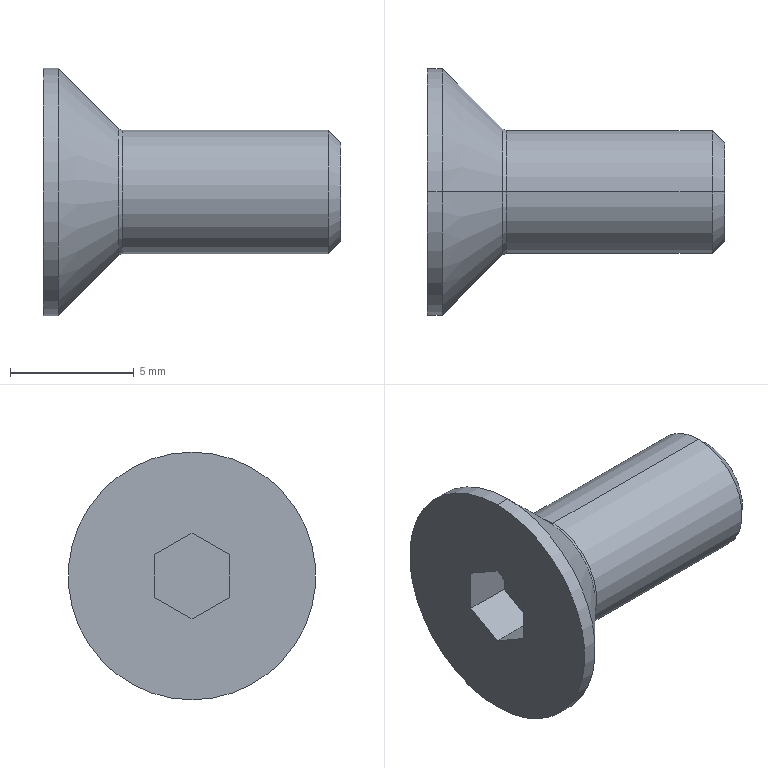Part | STEP file | 1 solid | 19 faces | box 12 x 10 x 10 mm | volume 319.784 mm3 | plane 9 | cone 4 | cylinder 4 | spline 2 | commonest cylinder face diameters 5 x2 10 x2
STEP:
#1=CARTESIAN_POINT('',(0.,0.,0.));
#2=DIRECTION('',(0.,0.,1.));
#3=DIRECTION('',(1.,0.,0.));
#4=AXIS2_PLACEMENT_3D('',#1,#2,#3);
#5=CARTESIAN_POINT('',(8.9,0.,2.));
#6=VERTEX_POINT('',#5);
#7=CARTESIAN_POINT('',(8.9,0.,-2.));
#8=VERTEX_POINT('',#7);
#9=CARTESIAN_POINT('',(8.9,0.,0.));
#10=DIRECTION('',(-1.,0.,0.));
#11=DIRECTION('',(0.,0.,1.));
#12=AXIS2_PLACEMENT_3D('',#9,#10,#11);
#13=CIRCLE('',#12,2.);
#14=CARTESIAN_POINT('',(8.9,2.5,0.));
#15=DIRECTION('',(-1.,0.,0.));
#16=DIRECTION('',(0.,0.,1.));
#17=AXIS2_PLACEMENT_3D('',#14,#15,#16);
#18=PLANE('',#17);
#19=CARTESIAN_POINT('',(0.,-2.5));
#20=DIRECTION('',(1.,0.));
#21=AXIS2_PLACEMENT_2D('',#19,#20);
#22=CIRCLE('',#21,2.);
#23=(GEOMETRIC_REPRESENTATION_CONTEXT(2)PARAMETRIC_REPRESENTATION_CONTEXT()REPRESENTATION_CONTEXT('',''));
#24=DEFINITIONAL_REPRESENTATION('',(#22),#23);
#25=PCURVE('',#18,#24);
#26=CARTESIAN_POINT('',(8.4,0.,0.));
#27=DIRECTION('',(-1.,0.,0.));
#28=DIRECTION('',(0.,0.,1.));
#29=AXIS2_PLACEMENT_3D('',#26,#27,#28);
#30=CONICAL_SURFACE('',#29,2.5,0.7854);
#31=CARTESIAN_POINT('',(0.,-0.5));
#32=DIRECTION('',(1.,0.));
#33=VECTOR('',#32,1.);
#34=LINE('',#31,#33);
#35=(GEOMETRIC_REPRESENTATION_CONTEXT(2)PARAMETRIC_REPRESENTATION_CONTEXT()REPRESENTATION_CONTEXT('',''));
#36=DEFINITIONAL_REPRESENTATION('',(#34),#35);
#37=PCURVE('',#30,#36);
#38=SURFACE_CURVE('',#13,(#25,#37),.PCURVE_S1.);
#39=EDGE_CURVE('',#6,#8,#38,.T.);
#40=ORIENTED_EDGE('',*,*,#39,.F.);
#41=CARTESIAN_POINT('',(8.9,0.,0.));
#42=DIRECTION('',(-1.,0.,0.));
#43=DIRECTION('',(0.,0.,1.));
#44=AXIS2_PLACEMENT_3D('',#41,#42,#43);
#45=CIRCLE('',#44,2.);
#46=CARTESIAN_POINT('',(0.,-2.5));
#47=DIRECTION('',(1.,0.));
#48=AXIS2_PLACEMENT_2D('',#46,#47);
#49=CIRCLE('',#48,2.);
#50=(GEOMETRIC_REPRESENTATION_CONTEXT(2)PARAMETRIC_REPRESENTATION_CONTEXT()REPRESENTATION_CONTEXT('',''));
#51=DEFINITIONAL_REPRESENTATION('',(#49),#50);
#52=PCURVE('',#18,#51);
#53=CARTESIAN_POINT('',(8.4,0.,0.));
#54=DIRECTION('',(-1.,0.,0.));
#55=DIRECTION('',(0.,0.,1.));
#56=AXIS2_PLACEMENT_3D('',#53,#54,#55);
#57=CONICAL_SURFACE('',#56,2.5,0.7854);
#58=CARTESIAN_POINT('',(0.,-0.5));
#59=DIRECTION('',(1.,0.));
#60=VECTOR('',#59,1.);
#61=LINE('',#58,#60);
#62=(GEOMETRIC_REPRESENTATION_CONTEXT(2)PARAMETRIC_REPRESENTATION_CONTEXT()REPRESENTATION_CONTEXT('',''));
#63=DEFINITIONAL_REPRESENTATION('',(#61),#62);
#64=PCURVE('',#57,#63);
#65=SURFACE_CURVE('',#45,(#52,#64),.PCURVE_S1.);
#66=EDGE_CURVE('',#8,#6,#65,.T.);
#67=ORIENTED_EDGE('',*,*,#66,.F.);
#68=EDGE_LOOP('',(#40,#67));
#69=FACE_BOUND('',#68,.T.);
#70=ADVANCED_FACE('',(#69),#18,.F.);
#71=CARTESIAN_POINT('',(8.4,0.,-2.5));
#72=VERTEX_POINT('',#71);
#73=CARTESIAN_POINT('',(8.4,0.,-2.5));
#74=DIRECTION('',(-0.7071,0.,-0.7071));
#75=VECTOR('',#74,1.);
#76=LINE('',#73,#75);
#77=CARTESIAN_POINT('',(3.142,0.));
#78=DIRECTION('',(0.,1.));
#79=VECTOR('',#78,1.);
#80=LINE('',#77,#79);
#81=(GEOMETRIC_REPRESENTATION_CONTEXT(2)PARAMETRIC_REPRESENTATION_CONTEXT()REPRESENTATION_CONTEXT('',''));
#82=DEFINITIONAL_REPRESENTATION('',(#80),#81);
#83=PCURVE('',#57,#82);
#84=CARTESIAN_POINT('',(3.142,0.));
#85=DIRECTION('',(0.,1.));
#86=VECTOR('',#85,1.);
#87=LINE('',#84,#86);
#88=(GEOMETRIC_REPRESENTATION_CONTEXT(2)PARAMETRIC_REPRESENTATION_CONTEXT()REPRESENTATION_CONTEXT('',''));
#89=DEFINITIONAL_REPRESENTATION('',(#87),#88);
#90=PCURVE('',#30,#89);
#91=SURFACE_CURVE('',#76,(#83,#90),.PCURVE_S1.);
#92=EDGE_CURVE('',#8,#72,#91,.T.);
#93=ORIENTED_EDGE('',*,*,#92,.F.);
#94=ORIENTED_EDGE('',*,*,#66,.T.);
#95=CARTESIAN_POINT('',(8.4,0.,2.5));
#96=VERTEX_POINT('',#95);
#97=CARTESIAN_POINT('',(8.4,0.,2.5));
#98=DIRECTION('',(-0.7071,0.,0.7071));
#99=VECTOR('',#98,1.);
#100=LINE('',#97,#99);
#101=CARTESIAN_POINT('',(6.283,0.));
#102=DIRECTION('',(0.,1.));
#103=VECTOR('',#102,1.);
#104=LINE('',#101,#103);
#105=(GEOMETRIC_REPRESENTATION_CONTEXT(2)PARAMETRIC_REPRESENTATION_CONTEXT()REPRESENTATION_CONTEXT('',''));
#106=DEFINITIONAL_REPRESENTATION('',(#104),#105);
#107=PCURVE('',#57,#106);
#108=CARTESIAN_POINT('',(0.,0.));
#109=DIRECTION('',(0.,1.));
#110=VECTOR('',#109,1.);
#111=LINE('',#108,#110);
#112=(GEOMETRIC_REPRESENTATION_CONTEXT(2)PARAMETRIC_REPRESENTATION_CONTEXT()REPRESENTATION_CONTEXT('',''));
#113=DEFINITIONAL_REPRESENTATION('',(#111),#112);
#114=PCURVE('',#30,#113);
#115=SURFACE_CURVE('',#100,(#107,#114),.PCURVE_S1.);
#116=EDGE_CURVE('',#6,#96,#115,.T.);
#117=ORIENTED_EDGE('',*,*,#116,.T.);
#118=CARTESIAN_POINT('',(8.4,0.,0.));
#119=DIRECTION('',(-1.,0.,0.));
#120=DIRECTION('',(0.,0.,1.));
#121=AXIS2_PLACEMENT_3D('',#118,#119,#120);
#122=CIRCLE('',#121,2.5);
#123=CARTESIAN_POINT('',(0.,0.));
#124=DIRECTION('',(1.,0.));
#125=VECTOR('',#124,1.);
#126=LINE('',#123,#125);
#127=(GEOMETRIC_REPRESENTATION_CONTEXT(2)PARAMETRIC_REPRESENTATION_CONTEXT()REPRESENTATION_CONTEXT('',''));
#128=DEFINITIONAL_REPRESENTATION('',(#126),#127);
#129=PCURVE('',#57,#128);
#130=CARTESIAN_POINT('',(-20.912,0.,0.));
#131=DIRECTION('',(-1.,0.,0.));
#132=DIRECTION('',(0.,0.,1.));
#133=AXIS2_PLACEMENT_3D('',#130,#131,#132);
#134=CYLINDRICAL_SURFACE('',#133,2.5);
#135=CARTESIAN_POINT('',(0.,-29.312));
#136=DIRECTION('',(1.,0.));
#137=VECTOR('',#136,1.);
#138=LINE('',#135,#137);
#139=(GEOMETRIC_REPRESENTATION_CONTEXT(2)PARAMETRIC_REPRESENTATION_CONTEXT()REPRESENTATION_CONTEXT('',''));
#140=DEFINITIONAL_REPRESENTATION('',(#138),#139);
#141=PCURVE('',#134,#140);
#142=SURFACE_CURVE('',#122,(#129,#141),.PCURVE_S1.);
#143=EDGE_CURVE('',#72,#96,#142,.T.);
#144=ORIENTED_EDGE('',*,*,#143,.F.);
#145=EDGE_LOOP('',(#93,#94,#117,#144));
#146=FACE_BOUND('',#145,.T.);
#147=ADVANCED_FACE('',(#146),#57,.T.);
#148=CARTESIAN_POINT('',(-3.1,-1.5,0.866));
#149=VERTEX_POINT('',#148);
#150=CARTESIAN_POINT('',(-1.2,-1.5,0.866));
#151=VERTEX_POINT('',#150);
#152=CARTESIAN_POINT('',(-1.2,-1.5,0.866));
#153=DIRECTION('',(1.,0.,0.));
#154=VECTOR('',#153,1.);
#155=LINE('',#152,#154);
#156=CARTESIAN_POINT('',(-1.2,-1.5,-0.866));
#157=DIRECTION('',(0.,-1.,0.));
#158=DIRECTION('',(-1.,0.,0.));
#159=AXIS2_PLACEMENT_3D('',#156,#157,#158);
#160=PLANE('',#159);
#161=CARTESIAN_POINT('',(0.,-1.732));
#162=DIRECTION('',(-1.,0.));
#163=VECTOR('',#162,1.);
#164=LINE('',#161,#163);
#165=(GEOMETRIC_REPRESENTATION_CONTEXT(2)PARAMETRIC_REPRESENTATION_CONTEXT()REPRESENTATION_CONTEXT('',''));
#166=DEFINITIONAL_REPRESENTATION('',(#164),#165);
#167=PCURVE('',#160,#166);
#168=CARTESIAN_POINT('',(-1.2,-1.5,0.866));
#169=DIRECTION('',(0.,-0.5,0.866));
#170=DIRECTION('',(-1.,0.,0.));
#171=AXIS2_PLACEMENT_3D('',#168,#169,#170);
#172=PLANE('',#171);
#173=CARTESIAN_POINT('',(0.,0.));
#174=DIRECTION('',(-1.,0.));
#175=VECTOR('',#174,1.);
#176=LINE('',#173,#175);
#177=(GEOMETRIC_REPRESENTATION_CONTEXT(2)PARAMETRIC_REPRESENTATION_CONTEXT()REPRESENTATION_CONTEXT('',''));
#178=DEFINITIONAL_REPRESENTATION('',(#176),#177);
#179=PCURVE('',#172,#178);
#180=SURFACE_CURVE('',#155,(#167,#179),.PCURVE_S1.);
#181=EDGE_CURVE('',#149,#151,#180,.T.);
#182=ORIENTED_EDGE('',*,*,#181,.T.);
#183=CARTESIAN_POINT('',(-1.2,-1.5,-0.866));
#184=VERTEX_POINT('',#183);
#185=CARTESIAN_POINT('',(-1.2,-1.5,-0.866));
#186=DIRECTION('',(0.,0.,1.));
#187=VECTOR('',#186,1.);
#188=LINE('',#185,#187);
#189=CARTESIAN_POINT('',(0.,0.));
#190=DIRECTION('',(0.,-1.));
#191=VECTOR('',#190,1.);
#192=LINE('',#189,#191);
#193=(GEOMETRIC_REPRESENTATION_CONTEXT(2)PARAMETRIC_REPRESENTATION_CONTEXT()REPRESENTATION_CONTEXT('',''));
#194=DEFINITIONAL_REPRESENTATION('',(#192),#193);
#195=PCURVE('',#160,#194);
#196=CARTESIAN_POINT('',(-1.2,0.,0.));
#197=DIRECTION('',(-1.,0.,0.));
#198=DIRECTION('',(0.,0.,1.));
#199=AXIS2_PLACEMENT_3D('',#196,#197,#198);
#200=PLANE('',#199);
#201=CARTESIAN_POINT('',(-0.866,-1.5));
#202=DIRECTION('',(1.,0.));
#203=VECTOR('',#202,1.);
#204=LINE('',#201,#203);
#205=(GEOMETRIC_REPRESENTATION_CONTEXT(2)PARAMETRIC_REPRESENTATION_CONTEXT()REPRESENTATION_CONTEXT('',''));
#206=DEFINITIONAL_REPRESENTATION('',(#204),#205);
#207=PCURVE('',#200,#206);
#208=SURFACE_CURVE('',#188,(#195,#207),.PCURVE_S1.);
#209=EDGE_CURVE('',#184,#151,#208,.T.);
#210=ORIENTED_EDGE('',*,*,#209,.F.);
#211=CARTESIAN_POINT('',(-3.1,-1.5,-0.866));
#212=VERTEX_POINT('',#211);
#213=CARTESIAN_POINT('',(-1.2,-1.5,-0.866));
#214=DIRECTION('',(-1.,0.,0.));
#215=VECTOR('',#214,1.);
#216=LINE('',#213,#215);
#217=CARTESIAN_POINT('',(0.,0.));
#218=DIRECTION('',(1.,0.));
#219=VECTOR('',#218,1.);
#220=LINE('',#217,#219);
#221=(GEOMETRIC_REPRESENTATION_CONTEXT(2)PARAMETRIC_REPRESENTATION_CONTEXT()REPRESENTATION_CONTEXT('',''));
#222=DEFINITIONAL_REPRESENTATION('',(#220),#221);
#223=PCURVE('',#160,#222);
#224=CARTESIAN_POINT('',(-1.2,0.,-1.732));
#225=DIRECTION('',(0.,-0.5,-0.866));
#226=DIRECTION('',(0.,-0.866,0.5));
#227=AXIS2_PLACEMENT_3D('',#224,#225,#226);
#228=PLANE('',#227);
#229=CARTESIAN_POINT('',(1.732,0.));
#230=DIRECTION('',(0.,1.));
#231=VECTOR('',#230,1.);
#232=LINE('',#229,#231);
#233=(GEOMETRIC_REPRESENTATION_CONTEXT(2)PARAMETRIC_REPRESENTATION_CONTEXT()REPRESENTATION_CONTEXT('',''));
#234=DEFINITIONAL_REPRESENTATION('',(#232),#233);
#235=PCURVE('',#228,#234);
#236=SURFACE_CURVE('',#216,(#223,#235),.PCURVE_S1.);
#237=EDGE_CURVE('',#184,#212,#236,.T.);
#238=ORIENTED_EDGE('',*,*,#237,.T.);
#239=CARTESIAN_POINT('',(-3.1,-1.5,-0.866));
#240=DIRECTION('',(0.,0.,-1.));
#241=VECTOR('',#240,1.);
#242=LINE('',#239,#241);
#243=CARTESIAN_POINT('',(1.9,0.));
#244=DIRECTION('',(0.,1.));
#245=VECTOR('',#244,1.);
#246=LINE('',#243,#245);
#247=(GEOMETRIC_REPRESENTATION_CONTEXT(2)PARAMETRIC_REPRESENTATION_CONTEXT()REPRESENTATION_CONTEXT('',''));
#248=DEFINITIONAL_REPRESENTATION('',(#246),#247);
#249=PCURVE('',#160,#248);
#250=CARTESIAN_POINT('',(-3.1,5.,0.));
#251=DIRECTION('',(1.,0.,0.));
#252=DIRECTION('',(0.,1.,0.));
#253=AXIS2_PLACEMENT_3D('',#250,#251,#252);
#254=PLANE('',#253);
#255=CARTESIAN_POINT('',(-6.5,-0.866));
#256=DIRECTION('',(0.,-1.));
#257=VECTOR('',#256,1.);
#258=LINE('',#255,#257);
#259=(GEOMETRIC_REPRESENTATION_CONTEXT(2)PARAMETRIC_REPRESENTATION_CONTEXT()REPRESENTATION_CONTEXT('',''));
#260=DEFINITIONAL_REPRESENTATION('',(#258),#259);
#261=PCURVE('',#254,#260);
#262=SURFACE_CURVE('',#242,(#249,#261),.PCURVE_S1.);
#263=EDGE_CURVE('',#149,#212,#262,.T.);
#264=ORIENTED_EDGE('',*,*,#263,.F.);
#265=EDGE_LOOP('',(#182,#210,#238,#264));
#266=FACE_BOUND('',#265,.T.);
#267=ADVANCED_FACE('',(#266),#160,.F.);
#268=CARTESIAN_POINT('',(0.08284,0.,-2.5));
#269=VERTEX_POINT('',#268);
#270=CARTESIAN_POINT('',(-20.912,0.,-2.5));
#271=DIRECTION('',(-1.,0.,0.));
#272=VECTOR('',#271,1.);
#273=LINE('',#270,#272);
#274=CARTESIAN_POINT('',(3.142,0.));
#275=DIRECTION('',(0.,1.));
#276=VECTOR('',#275,1.);
#277=LINE('',#274,#276);
#278=(GEOMETRIC_REPRESENTATION_CONTEXT(2)PARAMETRIC_REPRESENTATION_CONTEXT()REPRESENTATION_CONTEXT('',''));
#279=DEFINITIONAL_REPRESENTATION('',(#277),#278);
#280=PCURVE('',#134,#279);
#281=CARTESIAN_POINT('',(-20.912,0.,0.));
#282=DIRECTION('',(-1.,0.,0.));
#283=DIRECTION('',(0.,0.,1.));
#284=AXIS2_PLACEMENT_3D('',#281,#282,#283);
#285=CYLINDRICAL_SURFACE('',#284,2.5);
#286=CARTESIAN_POINT('',(3.142,0.));
#287=DIRECTION('',(0.,1.));
#288=VECTOR('',#287,1.);
#289=LINE('',#286,#288);
#290=(GEOMETRIC_REPRESENTATION_CONTEXT(2)PARAMETRIC_REPRESENTATION_CONTEXT()REPRESENTATION_CONTEXT('',''));
#291=DEFINITIONAL_REPRESENTATION('',(#289),#290);
#292=PCURVE('',#285,#291);
#293=SURFACE_CURVE('',#273,(#280,#292),.PCURVE_S1.);
#294=EDGE_CURVE('',#72,#269,#293,.T.);
#295=ORIENTED_EDGE('',*,*,#294,.F.);
#296=ORIENTED_EDGE('',*,*,#143,.T.);
#297=CARTESIAN_POINT('',(0.08284,0.,2.5));
#298=VERTEX_POINT('',#297);
#299=CARTESIAN_POINT('',(-20.912,0.,2.5));
#300=DIRECTION('',(-1.,0.,0.));
#301=VECTOR('',#300,1.);
#302=LINE('',#299,#301);
#303=CARTESIAN_POINT('',(6.283,0.));
#304=DIRECTION('',(0.,1.));
#305=VECTOR('',#304,1.);
#306=LINE('',#303,#305);
#307=(GEOMETRIC_REPRESENTATION_CONTEXT(2)PARAMETRIC_REPRESENTATION_CONTEXT()REPRESENTATION_CONTEXT('',''));
#308=DEFINITIONAL_REPRESENTATION('',(#306),#307);
#309=PCURVE('',#134,#308);
#310=CARTESIAN_POINT('',(0.,0.));
#311=DIRECTION('',(0.,1.));
#312=VECTOR('',#311,1.);
#313=LINE('',#310,#312);
#314=(GEOMETRIC_REPRESENTATION_CONTEXT(2)PARAMETRIC_REPRESENTATION_CONTEXT()REPRESENTATION_CONTEXT('',''));
#315=DEFINITIONAL_REPRESENTATION('',(#313),#314);
#316=PCURVE('',#285,#315);
#317=SURFACE_CURVE('',#302,(#309,#316),.PCURVE_S1.);
#318=EDGE_CURVE('',#96,#298,#317,.T.);
#319=ORIENTED_EDGE('',*,*,#318,.T.);
#320=CARTESIAN_POINT('',(0.08284,0.,0.));
#321=DIRECTION('',(1.,0.,0.));
#322=DIRECTION('',(0.,0.,1.));
#323=AXIS2_PLACEMENT_3D('',#320,#321,#322);
#324=CIRCLE('',#323,2.5);
#325=CARTESIAN_POINT('',(6.283,-20.995));
#326=DIRECTION('',(-1.,0.));
#327=VECTOR('',#326,1.);
#328=LINE('',#325,#327);
#329=(GEOMETRIC_REPRESENTATION_CONTEXT(2)PARAMETRIC_REPRESENTATION_CONTEXT()REPRESENTATION_CONTEXT('',''));
#330=DEFINITIONAL_REPRESENTATION('',(#328),#329);
#331=PCURVE('',#134,#330);
#332=CARTESIAN_POINT('',(0.08284,0.,-2.5));
#333=CARTESIAN_POINT('',(0.08284,-5.,-2.5));
#334=CARTESIAN_POINT('',(0.08284,-5.,2.5));
#335=CARTESIAN_POINT('',(0.08284,0.,2.5));
#336=CARTESIAN_POINT('',(0.02909,0.,-2.5));
#337=CARTESIAN_POINT('',(0.02909,-5.,-2.5));
#338=CARTESIAN_POINT('',(0.02909,-5.,2.5));
#339=CARTESIAN_POINT('',(0.02909,0.,2.5));
#340=CARTESIAN_POINT('',(-0.02057,0.,-2.521));
#341=CARTESIAN_POINT('',(-0.02057,-5.041,-2.521));
#342=CARTESIAN_POINT('',(-0.02057,-5.041,2.521));
#343=CARTESIAN_POINT('',(-0.02057,0.,2.521));
#344=CARTESIAN_POINT('',(-0.05858,0.,-2.559));
#345=CARTESIAN_POINT('',(-0.05858,-5.117,-2.559));
#346=CARTESIAN_POINT('',(-0.05858,-5.117,2.559));
#347=CARTESIAN_POINT('',(-0.05858,0.,2.559));
#348=(BOUNDED_SURFACE()B_SPLINE_SURFACE(3,3,((#332,#333,#334,#335),(#336,#337,#338,#339),(#340,#341,#342,#343),(#344,#345,#346,#347)),.UNSPECIFIED.,.F.,.F.,.F.)B_SPLINE_SURFACE_WITH_KNOTS((4,4),(4,4),(0.,1.),(0.,1.),.PIECEWISE_BEZIER_KNOTS.)GEOMETRIC_REPRESENTATION_ITEM()RATIONAL_B_SPLINE_SURFACE(((1.,0.3333,0.3333,1.),(0.9493,0.3164,0.3164,0.9493),(0.9493,0.3164,0.3164,0.9493),(1.,0.3333,0.3333,1.)))REPRESENTATION_ITEM('')SURFACE());
#349=CARTESIAN_POINT('',(0.,1.));
#350=CARTESIAN_POINT('',(0.,0.9763));
#351=CARTESIAN_POINT('',(0.,0.9319));
#352=CARTESIAN_POINT('',(0.,0.8733));
#353=CARTESIAN_POINT('',(0.,0.8206));
#354=CARTESIAN_POINT('',(0.,0.7724));
#355=CARTESIAN_POINT('',(0.,0.7279));
#356=CARTESIAN_POINT('',(0.,0.6861));
#357=CARTESIAN_POINT('',(0.,0.6465));
#358=CARTESIAN_POINT('',(0.,0.6086));
#359=CARTESIAN_POINT('',(0.,0.5718));
#360=CARTESIAN_POINT('',(0.,0.5357));
#361=CARTESIAN_POINT('',(0.,0.5));
#362=CARTESIAN_POINT('',(0.,0.4643));
#363=CARTESIAN_POINT('',(0.,0.4282));
#364=CARTESIAN_POINT('',(0.,0.3914));
#365=CARTESIAN_POINT('',(0.,0.3535));
#366=CARTESIAN_POINT('',(0.,0.3139));
#367=CARTESIAN_POINT('',(0.,0.2721));
#368=CARTESIAN_POINT('',(0.,0.2276));
#369=CARTESIAN_POINT('',(0.,0.1794));
#370=CARTESIAN_POINT('',(0.,0.1267));
#371=CARTESIAN_POINT('',(0.,0.06805));
#372=CARTESIAN_POINT('',(0.,0.02375));
#373=CARTESIAN_POINT('',(0.,0.));
#374=B_SPLINE_CURVE_WITH_KNOTS('',3,(#349,#350,#351,#352,#353,#354,#355,#356,#357,#358,#359,#360,#361,#362,#363,#364,#365,#366,#367,#368,#369,#370,#371,#372,#373),.UNSPECIFIED.,.F.,.F.,(4,1,1,1,1,1,1,1,1,1,1,1,1,1,1,1,1,1,1,1,1,1,4),(0.,0.1428,0.2856,0.4284,0.5712,0.714,0.8568,0.9996,1.142,1.285,1.428,1.571,1.714,1.856,1.999,2.142,2.285,2.428,2.57,2.713,2.856,2.999,3.142),.QUASI_UNIFORM_KNOTS.);
#375=(GEOMETRIC_REPRESENTATION_CONTEXT(2)PARAMETRIC_REPRESENTATION_CONTEXT()REPRESENTATION_CONTEXT('',''));
#376=DEFINITIONAL_REPRESENTATION('',(#374),#375);
#377=PCURVE('',#348,#376);
#378=SURFACE_CURVE('',#324,(#331,#377),.PCURVE_S1.);
#379=EDGE_CURVE('',#298,#269,#378,.T.);
#380=ORIENTED_EDGE('',*,*,#379,.T.);
#381=EDGE_LOOP('',(#295,#296,#319,#380));
#382=FACE_BOUND('',#381,.T.);
#383=ADVANCED_FACE('',(#382),#134,.T.);
#384=CARTESIAN_POINT('',(-3.1,0.,1.732));
#385=VERTEX_POINT('',#384);
#386=CARTESIAN_POINT('',(-1.2,0.,1.732));
#387=VERTEX_POINT('',#386);
#388=CARTESIAN_POINT('',(-1.2,0.,1.732));
#389=DIRECTION('',(1.,0.,0.));
#390=VECTOR('',#389,1.);
#391=LINE('',#388,#390);
#392=CARTESIAN_POINT('',(0.,-1.732));
#393=DIRECTION('',(-1.,0.));
#394=VECTOR('',#393,1.);
#395=LINE('',#392,#394);
#396=(GEOMETRIC_REPRESENTATION_CONTEXT(2)PARAMETRIC_REPRESENTATION_CONTEXT()REPRESENTATION_CONTEXT('',''));
#397=DEFINITIONAL_REPRESENTATION('',(#395),#396);
#398=PCURVE('',#172,#397);
#399=CARTESIAN_POINT('',(-1.2,0.,1.732));
#400=DIRECTION('',(0.,0.5,0.866));
#401=DIRECTION('',(1.,0.,0.));
#402=AXIS2_PLACEMENT_3D('',#399,#400,#401);
#403=PLANE('',#402);
#404=CARTESIAN_POINT('',(0.,0.));
#405=DIRECTION('',(1.,0.));
#406=VECTOR('',#405,1.);
#407=LINE('',#404,#406);
#408=(GEOMETRIC_REPRESENTATION_CONTEXT(2)PARAMETRIC_REPRESENTATION_CONTEXT()REPRESENTATION_CONTEXT('',''));
#409=DEFINITIONAL_REPRESENTATION('',(#407),#408);
#410=PCURVE('',#403,#409);
#411=SURFACE_CURVE('',#391,(#398,#410),.PCURVE_S1.);
#412=EDGE_CURVE('',#385,#387,#411,.T.);
#413=ORIENTED_EDGE('',*,*,#412,.T.);
#414=CARTESIAN_POINT('',(-1.2,-1.5,0.866));
#415=DIRECTION('',(0.,0.866,0.5));
#416=VECTOR('',#415,1.);
#417=LINE('',#414,#416);
#418=CARTESIAN_POINT('',(0.,0.));
#419=DIRECTION('',(0.,-1.));
#420=VECTOR('',#419,1.);
#421=LINE('',#418,#420);
#422=(GEOMETRIC_REPRESENTATION_CONTEXT(2)PARAMETRIC_REPRESENTATION_CONTEXT()REPRESENTATION_CONTEXT('',''));
#423=DEFINITIONAL_REPRESENTATION('',(#421),#422);
#424=PCURVE('',#172,#423);
#425=CARTESIAN_POINT('',(0.866,-1.5));
#426=DIRECTION('',(0.5,0.866));
#427=VECTOR('',#426,1.);
#428=LINE('',#425,#427);
#429=(GEOMETRIC_REPRESENTATION_CONTEXT(2)PARAMETRIC_REPRESENTATION_CONTEXT()REPRESENTATION_CONTEXT('',''));
#430=DEFINITIONAL_REPRESENTATION('',(#428),#429);
#431=PCURVE('',#200,#430);
#432=SURFACE_CURVE('',#417,(#424,#431),.PCURVE_S1.);
#433=EDGE_CURVE('',#151,#387,#432,.T.);
#434=ORIENTED_EDGE('',*,*,#433,.F.);
#435=ORIENTED_EDGE('',*,*,#181,.F.);
#436=CARTESIAN_POINT('',(-3.1,-1.5,0.866));
#437=DIRECTION('',(0.,-0.866,-0.5));
#438=VECTOR('',#437,1.);
#439=LINE('',#436,#438);
#440=CARTESIAN_POINT('',(1.9,0.));
#441=DIRECTION('',(0.,1.));
#442=VECTOR('',#441,1.);
#443=LINE('',#440,#442);
#444=(GEOMETRIC_REPRESENTATION_CONTEXT(2)PARAMETRIC_REPRESENTATION_CONTEXT()REPRESENTATION_CONTEXT('',''));
#445=DEFINITIONAL_REPRESENTATION('',(#443),#444);
#446=PCURVE('',#172,#445);
#447=CARTESIAN_POINT('',(-6.5,0.866));
#448=DIRECTION('',(-0.866,-0.5));
#449=VECTOR('',#448,1.);
#450=LINE('',#447,#449);
#451=(GEOMETRIC_REPRESENTATION_CONTEXT(2)PARAMETRIC_REPRESENTATION_CONTEXT()REPRESENTATION_CONTEXT('',''));
#452=DEFINITIONAL_REPRESENTATION('',(#450),#451);
#453=PCURVE('',#254,#452);
#454=SURFACE_CURVE('',#439,(#446,#453),.PCURVE_S1.);
#455=EDGE_CURVE('',#385,#149,#454,.T.);
#456=ORIENTED_EDGE('',*,*,#455,.F.);
#457=EDGE_LOOP('',(#413,#434,#435,#456));
#458=FACE_BOUND('',#457,.T.);
#459=ADVANCED_FACE('',(#458),#172,.F.);
#460=ORIENTED_EDGE('',*,*,#237,.F.);
#461=CARTESIAN_POINT('',(-1.2,0.,-1.732));
#462=VERTEX_POINT('',#461);
#463=CARTESIAN_POINT('',(-1.2,0.,-1.732));
#464=DIRECTION('',(0.,-0.866,0.5));
#465=VECTOR('',#464,1.);
#466=LINE('',#463,#465);
#467=CARTESIAN_POINT('',(0.,0.));
#468=DIRECTION('',(1.,0.));
#469=VECTOR('',#468,1.);
#470=LINE('',#467,#469);
#471=(GEOMETRIC_REPRESENTATION_CONTEXT(2)PARAMETRIC_REPRESENTATION_CONTEXT()REPRESENTATION_CONTEXT('',''));
#472=DEFINITIONAL_REPRESENTATION('',(#470),#471);
#473=PCURVE('',#228,#472);
#474=CARTESIAN_POINT('',(-1.732,0.));
#475=DIRECTION('',(0.5,-0.866));
#476=VECTOR('',#475,1.);
#477=LINE('',#474,#476);
#478=(GEOMETRIC_REPRESENTATION_CONTEXT(2)PARAMETRIC_REPRESENTATION_CONTEXT()REPRESENTATION_CONTEXT('',''));
#479=DEFINITIONAL_REPRESENTATION('',(#477),#478);
#480=PCURVE('',#200,#479);
#481=SURFACE_CURVE('',#466,(#473,#480),.PCURVE_S1.);
#482=EDGE_CURVE('',#462,#184,#481,.T.);
#483=ORIENTED_EDGE('',*,*,#482,.F.);
#484=CARTESIAN_POINT('',(-3.1,0.,-1.732));
#485=VERTEX_POINT('',#484);
#486=CARTESIAN_POINT('',(-1.2,0.,-1.732));
#487=DIRECTION('',(-1.,0.,0.));
#488=VECTOR('',#487,1.);
#489=LINE('',#486,#488);
#490=CARTESIAN_POINT('',(0.,0.));
#491=DIRECTION('',(0.,1.));
#492=VECTOR('',#491,1.);
#493=LINE('',#490,#492);
#494=(GEOMETRIC_REPRESENTATION_CONTEXT(2)PARAMETRIC_REPRESENTATION_CONTEXT()REPRESENTATION_CONTEXT('',''));
#495=DEFINITIONAL_REPRESENTATION('',(#493),#494);
#496=PCURVE('',#228,#495);
#497=CARTESIAN_POINT('',(-1.2,1.5,-0.866));
#498=DIRECTION('',(0.,0.5,-0.866));
#499=DIRECTION('',(-1.,0.,0.));
#500=AXIS2_PLACEMENT_3D('',#497,#498,#499);
#501=PLANE('',#500);
#502=CARTESIAN_POINT('',(0.,-1.732));
#503=DIRECTION('',(1.,0.));
#504=VECTOR('',#503,1.);
#505=LINE('',#502,#504);
#506=(GEOMETRIC_REPRESENTATION_CONTEXT(2)PARAMETRIC_REPRESENTATION_CONTEXT()REPRESENTATION_CONTEXT('',''));
#507=DEFINITIONAL_REPRESENTATION('',(#505),#506);
#508=PCURVE('',#501,#507);
#509=SURFACE_CURVE('',#489,(#496,#508),.PCURVE_S1.);
#510=EDGE_CURVE('',#462,#485,#509,.T.);
#511=ORIENTED_EDGE('',*,*,#510,.T.);
#512=CARTESIAN_POINT('',(-3.1,0.,-1.732));
#513=DIRECTION('',(0.,0.866,-0.5));
#514=VECTOR('',#513,1.);
#515=LINE('',#512,#514);
#516=CARTESIAN_POINT('',(0.,1.9));
#517=DIRECTION('',(-1.,0.));
#518=VECTOR('',#517,1.);
#519=LINE('',#516,#518);
#520=(GEOMETRIC_REPRESENTATION_CONTEXT(2)PARAMETRIC_REPRESENTATION_CONTEXT()REPRESENTATION_CONTEXT('',''));
#521=DEFINITIONAL_REPRESENTATION('',(#519),#520);
#522=PCURVE('',#228,#521);
#523=CARTESIAN_POINT('',(-5.,-1.732));
#524=DIRECTION('',(0.866,-0.5));
#525=VECTOR('',#524,1.);
#526=LINE('',#523,#525);
#527=(GEOMETRIC_REPRESENTATION_CONTEXT(2)PARAMETRIC_REPRESENTATION_CONTEXT()REPRESENTATION_CONTEXT('',''));
#528=DEFINITIONAL_REPRESENTATION('',(#526),#527);
#529=PCURVE('',#254,#528);
#530=SURFACE_CURVE('',#515,(#522,#529),.PCURVE_S1.);
#531=EDGE_CURVE('',#212,#485,#530,.T.);
#532=ORIENTED_EDGE('',*,*,#531,.F.);
#533=EDGE_LOOP('',(#460,#483,#511,#532));
#534=FACE_BOUND('',#533,.T.);
#535=ADVANCED_FACE('',(#534),#228,.F.);
#536=CARTESIAN_POINT('',(-0.05858,0.,-2.559));
#537=VERTEX_POINT('',#536);
#538=CARTESIAN_POINT('',(-0.05858,0.,2.559));
#539=VERTEX_POINT('',#538);
#540=CARTESIAN_POINT('',(-0.05858,0.,0.));
#541=DIRECTION('',(-1.,0.,0.));
#542=DIRECTION('',(0.,0.,1.));
#543=AXIS2_PLACEMENT_3D('',#540,#541,#542);
#544=CIRCLE('',#543,2.559);
#545=CARTESIAN_POINT('',(1.,0.));
#546=CARTESIAN_POINT('',(1.,0.02375));
#547=CARTESIAN_POINT('',(1.,0.06805));
#548=CARTESIAN_POINT('',(1.,0.1267));
#549=CARTESIAN_POINT('',(1.,0.1794));
#550=CARTESIAN_POINT('',(1.,0.2276));
#551=CARTESIAN_POINT('',(1.,0.2721));
#552=CARTESIAN_POINT('',(1.,0.3139));
#553=CARTESIAN_POINT('',(1.,0.3535));
#554=CARTESIAN_POINT('',(1.,0.3914));
#555=CARTESIAN_POINT('',(1.,0.4282));
#556=CARTESIAN_POINT('',(1.,0.4643));
#557=CARTESIAN_POINT('',(1.,0.5));
#558=CARTESIAN_POINT('',(1.,0.5357));
#559=CARTESIAN_POINT('',(1.,0.5718));
#560=CARTESIAN_POINT('',(1.,0.6086));
#561=CARTESIAN_POINT('',(1.,0.6465));
#562=CARTESIAN_POINT('',(1.,0.6861));
#563=CARTESIAN_POINT('',(1.,0.7279));
#564=CARTESIAN_POINT('',(1.,0.7724));
#565=CARTESIAN_POINT('',(1.,0.8206));
#566=CARTESIAN_POINT('',(1.,0.8733));
#567=CARTESIAN_POINT('',(1.,0.9319));
#568=CARTESIAN_POINT('',(1.,0.9763));
#569=CARTESIAN_POINT('',(1.,1.));
#570=B_SPLINE_CURVE_WITH_KNOTS('',3,(#545,#546,#547,#548,#549,#550,#551,#552,#553,#554,#555,#556,#557,#558,#559,#560,#561,#562,#563,#564,#565,#566,#567,#568,#569),.UNSPECIFIED.,.F.,.F.,(4,1,1,1,1,1,1,1,1,1,1,1,1,1,1,1,1,1,1,1,1,1,4),(3.142,3.284,3.427,3.57,3.713,3.856,3.998,4.141,4.284,4.427,4.57,4.712,4.855,4.998,5.141,5.284,5.426,5.569,5.712,5.855,5.998,6.14,6.283),.QUASI_UNIFORM_KNOTS.);
#571=(GEOMETRIC_REPRESENTATION_CONTEXT(2)PARAMETRIC_REPRESENTATION_CONTEXT()REPRESENTATION_CONTEXT('',''));
#572=DEFINITIONAL_REPRESENTATION('',(#570),#571);
#573=PCURVE('',#348,#572);
#574=CARTESIAN_POINT('',(-2.5,0.,0.));
#575=DIRECTION('',(-1.,0.,0.));
#576=DIRECTION('',(0.,0.,1.));
#577=AXIS2_PLACEMENT_3D('',#574,#575,#576);
#578=CONICAL_SURFACE('',#577,5.,0.7854);
#579=CARTESIAN_POINT('',(0.,-2.441));
#580=DIRECTION('',(1.,0.));
#581=VECTOR('',#580,1.);
#582=LINE('',#579,#581);
#583=(GEOMETRIC_REPRESENTATION_CONTEXT(2)PARAMETRIC_REPRESENTATION_CONTEXT()REPRESENTATION_CONTEXT('',''));
#584=DEFINITIONAL_REPRESENTATION('',(#582),#583);
#585=PCURVE('',#578,#584);
#586=SURFACE_CURVE('',#544,(#573,#585),.PCURVE_S1.);
#587=EDGE_CURVE('',#537,#539,#586,.T.);
#588=ORIENTED_EDGE('',*,*,#587,.T.);
#589=CARTESIAN_POINT('',(0.08284,0.,2.7));
#590=DIRECTION('',(0.,1.,0.));
#591=DIRECTION('',(0.,0.,1.));
#592=AXIS2_PLACEMENT_3D('',#589,#590,#591);
#593=CIRCLE('',#592,0.2);
#594=CARTESIAN_POINT('',(0.,1.));
#595=CARTESIAN_POINT('',(0.01555,1.));
#596=CARTESIAN_POINT('',(0.04653,1.));
#597=CARTESIAN_POINT('',(0.09271,1.));
#598=CARTESIAN_POINT('',(0.1386,1.));
#599=CARTESIAN_POINT('',(0.1843,1.));
#600=CARTESIAN_POINT('',(0.2298,1.));
#601=CARTESIAN_POINT('',(0.2751,1.));
#602=CARTESIAN_POINT('',(0.3202,1.));
#603=CARTESIAN_POINT('',(0.3653,1.));
#604=CARTESIAN_POINT('',(0.4102,1.));
#605=CARTESIAN_POINT('',(0.4551,1.));
#606=CARTESIAN_POINT('',(0.5,1.));
#607=CARTESIAN_POINT('',(0.5449,1.));
#608=CARTESIAN_POINT('',(0.5898,1.));
#609=CARTESIAN_POINT('',(0.6347,1.));
#610=CARTESIAN_POINT('',(0.6798,1.));
#611=CARTESIAN_POINT('',(0.7249,1.));
#612=CARTESIAN_POINT('',(0.7702,1.));
#613=CARTESIAN_POINT('',(0.8157,1.));
#614=CARTESIAN_POINT('',(0.8614,1.));
#615=CARTESIAN_POINT('',(0.9073,1.));
#616=CARTESIAN_POINT('',(0.9535,1.));
#617=CARTESIAN_POINT('',(0.9845,1.));
#618=CARTESIAN_POINT('',(1.,1.));
#619=B_SPLINE_CURVE_WITH_KNOTS('',3,(#594,#595,#596,#597,#598,#599,#600,#601,#602,#603,#604,#605,#606,#607,#608,#609,#610,#611,#612,#613,#614,#615,#616,#617,#618),.UNSPECIFIED.,.F.,.F.,(4,1,1,1,1,1,1,1,1,1,1,1,1,1,1,1,1,1,1,1,1,1,4),(3.142,3.177,3.213,3.249,3.284,3.32,3.356,3.391,3.427,3.463,3.499,3.534,3.57,3.606,3.641,3.677,3.713,3.748,3.784,3.82,3.856,3.891,3.927),.QUASI_UNIFORM_KNOTS.);
#620=(GEOMETRIC_REPRESENTATION_CONTEXT(2)PARAMETRIC_REPRESENTATION_CONTEXT()REPRESENTATION_CONTEXT('',''));
#621=DEFINITIONAL_REPRESENTATION('',(#619),#620);
#622=PCURVE('',#348,#621);
#623=CARTESIAN_POINT('',(0.08284,0.,2.5));
#624=CARTESIAN_POINT('',(0.08284,5.,2.5));
#625=CARTESIAN_POINT('',(0.08284,5.,-2.5));
#626=CARTESIAN_POINT('',(0.08284,0.,-2.5));
#627=CARTESIAN_POINT('',(0.02909,0.,2.5));
#628=CARTESIAN_POINT('',(0.02909,5.,2.5));
#629=CARTESIAN_POINT('',(0.02909,5.,-2.5));
#630=CARTESIAN_POINT('',(0.02909,0.,-2.5));
#631=CARTESIAN_POINT('',(-0.02057,0.,2.521));
#632=CARTESIAN_POINT('',(-0.02057,5.041,2.521));
#633=CARTESIAN_POINT('',(-0.02057,5.041,-2.521));
#634=CARTESIAN_POINT('',(-0.02057,0.,-2.521));
#635=CARTESIAN_POINT('',(-0.05858,0.,2.559));
#636=CARTESIAN_POINT('',(-0.05858,5.117,2.559));
#637=CARTESIAN_POINT('',(-0.05858,5.117,-2.559));
#638=CARTESIAN_POINT('',(-0.05858,0.,-2.559));
#639=(BOUNDED_SURFACE()B_SPLINE_SURFACE(3,3,((#623,#624,#625,#626),(#627,#628,#629,#630),(#631,#632,#633,#634),(#635,#636,#637,#638)),.UNSPECIFIED.,.F.,.F.,.F.)B_SPLINE_SURFACE_WITH_KNOTS((4,4),(4,4),(0.,1.),(0.,1.),.PIECEWISE_BEZIER_KNOTS.)GEOMETRIC_REPRESENTATION_ITEM()RATIONAL_B_SPLINE_SURFACE(((1.,0.3333,0.3333,1.),(0.9493,0.3164,0.3164,0.9493),(0.9493,0.3164,0.3164,0.9493),(1.,0.3333,0.3333,1.)))REPRESENTATION_ITEM('')SURFACE());
#640=CARTESIAN_POINT('',(0.,0.));
#641=CARTESIAN_POINT('',(0.01555,0.));
#642=CARTESIAN_POINT('',(0.04653,0.));
#643=CARTESIAN_POINT('',(0.09271,0.));
#644=CARTESIAN_POINT('',(0.1386,0.));
#645=CARTESIAN_POINT('',(0.1843,0.));
#646=CARTESIAN_POINT('',(0.2298,0.));
#647=CARTESIAN_POINT('',(0.2751,0.));
#648=CARTESIAN_POINT('',(0.3202,0.));
#649=CARTESIAN_POINT('',(0.3653,0.));
#650=CARTESIAN_POINT('',(0.4102,0.));
#651=CARTESIAN_POINT('',(0.4551,0.));
#652=CARTESIAN_POINT('',(0.5,0.));
#653=CARTESIAN_POINT('',(0.5449,0.));
#654=CARTESIAN_POINT('',(0.5898,0.));
#655=CARTESIAN_POINT('',(0.6347,0.));
#656=CARTESIAN_POINT('',(0.6798,0.));
#657=CARTESIAN_POINT('',(0.7249,0.));
#658=CARTESIAN_POINT('',(0.7702,0.));
#659=CARTESIAN_POINT('',(0.8157,0.));
#660=CARTESIAN_POINT('',(0.8614,0.));
#661=CARTESIAN_POINT('',(0.9073,0.));
#662=CARTESIAN_POINT('',(0.9535,0.));
#663=CARTESIAN_POINT('',(0.9845,0.));
#664=CARTESIAN_POINT('',(1.,0.));
#665=B_SPLINE_CURVE_WITH_KNOTS('',3,(#640,#641,#642,#643,#644,#645,#646,#647,#648,#649,#650,#651,#652,#653,#654,#655,#656,#657,#658,#659,#660,#661,#662,#663,#664),.UNSPECIFIED.,.F.,.F.,(4,1,1,1,1,1,1,1,1,1,1,1,1,1,1,1,1,1,1,1,1,1,4),(3.142,3.177,3.213,3.249,3.284,3.32,3.356,3.391,3.427,3.463,3.499,3.534,3.57,3.606,3.641,3.677,3.713,3.748,3.784,3.82,3.856,3.891,3.927),.QUASI_UNIFORM_KNOTS.);
#666=(GEOMETRIC_REPRESENTATION_CONTEXT(2)PARAMETRIC_REPRESENTATION_CONTEXT()REPRESENTATION_CONTEXT('',''));
#667=DEFINITIONAL_REPRESENTATION('',(#665),#666);
#668=PCURVE('',#639,#667);
#669=SURFACE_CURVE('',#593,(#622,#668),.PCURVE_S1.);
#670=EDGE_CURVE('',#298,#539,#669,.T.);
#671=ORIENTED_EDGE('',*,*,#670,.F.);
#672=ORIENTED_EDGE('',*,*,#379,.T.);
#673=CARTESIAN_POINT('',(0.08284,0.,-2.7));
#674=DIRECTION('',(0.,-1.,0.));
#675=DIRECTION('',(0.,0.,-1.));
#676=AXIS2_PLACEMENT_3D('',#673,#674,#675);
#677=CIRCLE('',#676,0.2);
#678=CARTESIAN_POINT('',(0.,0.));
#679=CARTESIAN_POINT('',(0.01555,0.));
#680=CARTESIAN_POINT('',(0.04653,0.));
#681=CARTESIAN_POINT('',(0.09271,0.));
#682=CARTESIAN_POINT('',(0.1386,0.));
#683=CARTESIAN_POINT('',(0.1843,0.));
#684=CARTESIAN_POINT('',(0.2298,0.));
#685=CARTESIAN_POINT('',(0.2751,0.));
#686=CARTESIAN_POINT('',(0.3202,0.));
#687=CARTESIAN_POINT('',(0.3653,0.));
#688=CARTESIAN_POINT('',(0.4102,0.));
#689=CARTESIAN_POINT('',(0.4551,0.));
#690=CARTESIAN_POINT('',(0.5,0.));
#691=CARTESIAN_POINT('',(0.5449,0.));
#692=CARTESIAN_POINT('',(0.5898,0.));
#693=CARTESIAN_POINT('',(0.6347,0.));
#694=CARTESIAN_POINT('',(0.6798,0.));
#695=CARTESIAN_POINT('',(0.7249,0.));
#696=CARTESIAN_POINT('',(0.7702,0.));
#697=CARTESIAN_POINT('',(0.8157,0.));
#698=CARTESIAN_POINT('',(0.8614,0.));
#699=CARTESIAN_POINT('',(0.9073,0.));
#700=CARTESIAN_POINT('',(0.9535,0.));
#701=CARTESIAN_POINT('',(0.9845,0.));
#702=CARTESIAN_POINT('',(1.,0.));
#703=B_SPLINE_CURVE_WITH_KNOTS('',3,(#678,#679,#680,#681,#682,#683,#684,#685,#686,#687,#688,#689,#690,#691,#692,#693,#694,#695,#696,#697,#698,#699,#700,#701,#702),.UNSPECIFIED.,.F.,.F.,(4,1,1,1,1,1,1,1,1,1,1,1,1,1,1,1,1,1,1,1,1,1,4),(3.142,3.177,3.213,3.249,3.284,3.32,3.356,3.391,3.427,3.463,3.499,3.534,3.57,3.606,3.641,3.677,3.713,3.748,3.784,3.82,3.856,3.891,3.927),.QUASI_UNIFORM_KNOTS.);
#704=(GEOMETRIC_REPRESENTATION_CONTEXT(2)PARAMETRIC_REPRESENTATION_CONTEXT()REPRESENTATION_CONTEXT('',''));
#705=DEFINITIONAL_REPRESENTATION('',(#703),#704);
#706=PCURVE('',#348,#705);
#707=CARTESIAN_POINT('',(0.,1.));
#708=CARTESIAN_POINT('',(0.01555,1.));
#709=CARTESIAN_POINT('',(0.04653,1.));
#710=CARTESIAN_POINT('',(0.09271,1.));
#711=CARTESIAN_POINT('',(0.1386,1.));
#712=CARTESIAN_POINT('',(0.1843,1.));
#713=CARTESIAN_POINT('',(0.2298,1.));
#714=CARTESIAN_POINT('',(0.2751,1.));
#715=CARTESIAN_POINT('',(0.3202,1.));
#716=CARTESIAN_POINT('',(0.3653,1.));
#717=CARTESIAN_POINT('',(0.4102,1.));
#718=CARTESIAN_POINT('',(0.4551,1.));
#719=CARTESIAN_POINT('',(0.5,1.));
#720=CARTESIAN_POINT('',(0.5449,1.));
#721=CARTESIAN_POINT('',(0.5898,1.));
#722=CARTESIAN_POINT('',(0.6347,1.));
#723=CARTESIAN_POINT('',(0.6798,1.));
#724=CARTESIAN_POINT('',(0.7249,1.));
#725=CARTESIAN_POINT('',(0.7702,1.));
#726=CARTESIAN_POINT('',(0.8157,1.));
#727=CARTESIAN_POINT('',(0.8614,1.));
#728=CARTESIAN_POINT('',(0.9073,1.));
#729=CARTESIAN_POINT('',(0.9535,1.));
#730=CARTESIAN_POINT('',(0.9845,1.));
#731=CARTESIAN_POINT('',(1.,1.));
#732=B_SPLINE_CURVE_WITH_KNOTS('',3,(#707,#708,#709,#710,#711,#712,#713,#714,#715,#716,#717,#718,#719,#720,#721,#722,#723,#724,#725,#726,#727,#728,#729,#730,#731),.UNSPECIFIED.,.F.,.F.,(4,1,1,1,1,1,1,1,1,1,1,1,1,1,1,1,1,1,1,1,1,1,4),(3.142,3.177,3.213,3.249,3.284,3.32,3.356,3.391,3.427,3.463,3.499,3.534,3.57,3.606,3.641,3.677,3.713,3.748,3.784,3.82,3.856,3.891,3.927),.QUASI_UNIFORM_KNOTS.);
#733=(GEOMETRIC_REPRESENTATION_CONTEXT(2)PARAMETRIC_REPRESENTATION_CONTEXT()REPRESENTATION_CONTEXT('',''));
#734=DEFINITIONAL_REPRESENTATION('',(#732),#733);
#735=PCURVE('',#639,#734);
#736=SURFACE_CURVE('',#677,(#706,#735),.PCURVE_S1.);
#737=EDGE_CURVE('',#269,#537,#736,.T.);
#738=ORIENTED_EDGE('',*,*,#737,.T.);
#739=EDGE_LOOP('',(#588,#671,#672,#738));
#740=FACE_BOUND('',#739,.F.);
#741=ADVANCED_FACE('',(#740),#348,.F.);
#742=CARTESIAN_POINT('',(-3.1,1.5,0.866));
#743=VERTEX_POINT('',#742);
#744=CARTESIAN_POINT('',(-1.2,1.5,0.866));
#745=VERTEX_POINT('',#744);
#746=CARTESIAN_POINT('',(-1.2,1.5,0.866));
#747=DIRECTION('',(1.,0.,0.));
#748=VECTOR('',#747,1.);
#749=LINE('',#746,#748);
#750=CARTESIAN_POINT('',(0.,1.732));
#751=DIRECTION('',(1.,0.));
#752=VECTOR('',#751,1.);
#753=LINE('',#750,#752);
#754=(GEOMETRIC_REPRESENTATION_CONTEXT(2)PARAMETRIC_REPRESENTATION_CONTEXT()REPRESENTATION_CONTEXT('',''));
#755=DEFINITIONAL_REPRESENTATION('',(#753),#754);
#756=PCURVE('',#403,#755);
#757=CARTESIAN_POINT('',(-1.2,1.5,0.866));
#758=DIRECTION('',(0.,1.,0.));
#759=DIRECTION('',(1.,0.,0.));
#760=AXIS2_PLACEMENT_3D('',#757,#758,#759);
#761=PLANE('',#760);
#762=CARTESIAN_POINT('',(0.,0.));
#763=DIRECTION('',(1.,0.));
#764=VECTOR('',#763,1.);
#765=LINE('',#762,#764);
#766=(GEOMETRIC_REPRESENTATION_CONTEXT(2)PARAMETRIC_REPRESENTATION_CONTEXT()REPRESENTATION_CONTEXT('',''));
#767=DEFINITIONAL_REPRESENTATION('',(#765),#766);
#768=PCURVE('',#761,#767);
#769=SURFACE_CURVE('',#749,(#756,#768),.PCURVE_S1.);
#770=EDGE_CURVE('',#743,#745,#769,.T.);
#771=ORIENTED_EDGE('',*,*,#770,.T.);
#772=CARTESIAN_POINT('',(-1.2,0.,1.732));
#773=DIRECTION('',(0.,0.866,-0.5));
#774=VECTOR('',#773,1.);
#775=LINE('',#772,#774);
#776=CARTESIAN_POINT('',(0.,0.));
#777=DIRECTION('',(0.,1.));
#778=VECTOR('',#777,1.);
#779=LINE('',#776,#778);
#780=(GEOMETRIC_REPRESENTATION_CONTEXT(2)PARAMETRIC_REPRESENTATION_CONTEXT()REPRESENTATION_CONTEXT('',''));
#781=DEFINITIONAL_REPRESENTATION('',(#779),#780);
#782=PCURVE('',#403,#781);
#783=CARTESIAN_POINT('',(1.732,0.));
#784=DIRECTION('',(-0.5,0.866));
#785=VECTOR('',#784,1.);
#786=LINE('',#783,#785);
#787=(GEOMETRIC_REPRESENTATION_CONTEXT(2)PARAMETRIC_REPRESENTATION_CONTEXT()REPRESENTATION_CONTEXT('',''));
#788=DEFINITIONAL_REPRESENTATION('',(#786),#787);
#789=PCURVE('',#200,#788);
#790=SURFACE_CURVE('',#775,(#782,#789),.PCURVE_S1.);
#791=EDGE_CURVE('',#387,#745,#790,.T.);
#792=ORIENTED_EDGE('',*,*,#791,.F.);
#793=ORIENTED_EDGE('',*,*,#412,.F.);
#794=CARTESIAN_POINT('',(-3.1,0.,1.732));
#795=DIRECTION('',(0.,-0.866,0.5));
#796=VECTOR('',#795,1.);
#797=LINE('',#794,#796);
#798=CARTESIAN_POINT('',(-1.9,0.));
#799=DIRECTION('',(0.,-1.));
#800=VECTOR('',#799,1.);
#801=LINE('',#798,#800);
#802=(GEOMETRIC_REPRESENTATION_CONTEXT(2)PARAMETRIC_REPRESENTATION_CONTEXT()REPRESENTATION_CONTEXT('',''));
#803=DEFINITIONAL_REPRESENTATION('',(#801),#802);
#804=PCURVE('',#403,#803);
#805=CARTESIAN_POINT('',(-5.,1.732));
#806=DIRECTION('',(-0.866,0.5));
#807=VECTOR('',#806,1.);
#808=LINE('',#805,#807);
#809=(GEOMETRIC_REPRESENTATION_CONTEXT(2)PARAMETRIC_REPRESENTATION_CONTEXT()REPRESENTATION_CONTEXT('',''));
#810=DEFINITIONAL_REPRESENTATION('',(#808),#809);
#811=PCURVE('',#254,#810);
#812=SURFACE_CURVE('',#797,(#804,#811),.PCURVE_S1.);
#813=EDGE_CURVE('',#743,#385,#812,.T.);
#814=ORIENTED_EDGE('',*,*,#813,.F.);
#815=EDGE_LOOP('',(#771,#792,#793,#814));
#816=FACE_BOUND('',#815,.T.);
#817=ADVANCED_FACE('',(#816),#403,.F.);
#818=ORIENTED_EDGE('',*,*,#209,.T.);
#819=ORIENTED_EDGE('',*,*,#433,.T.);
#820=ORIENTED_EDGE('',*,*,#791,.T.);
#821=CARTESIAN_POINT('',(-1.2,1.5,-0.866));
#822=VERTEX_POINT('',#821);
#823=CARTESIAN_POINT('',(-1.2,1.5,0.866));
#824=DIRECTION('',(0.,0.,-1.));
#825=VECTOR('',#824,1.);
#826=LINE('',#823,#825);
#827=CARTESIAN_POINT('',(0.866,1.5));
#828=DIRECTION('',(-1.,0.));
#829=VECTOR('',#828,1.);
#830=LINE('',#827,#829);
#831=(GEOMETRIC_REPRESENTATION_CONTEXT(2)PARAMETRIC_REPRESENTATION_CONTEXT()REPRESENTATION_CONTEXT('',''));
#832=DEFINITIONAL_REPRESENTATION('',(#830),#831);
#833=PCURVE('',#200,#832);
#834=CARTESIAN_POINT('',(0.,0.));
#835=DIRECTION('',(0.,1.));
#836=VECTOR('',#835,1.);
#837=LINE('',#834,#836);
#838=(GEOMETRIC_REPRESENTATION_CONTEXT(2)PARAMETRIC_REPRESENTATION_CONTEXT()REPRESENTATION_CONTEXT('',''));
#839=DEFINITIONAL_REPRESENTATION('',(#837),#838);
#840=PCURVE('',#761,#839);
#841=SURFACE_CURVE('',#826,(#833,#840),.PCURVE_S1.);
#842=EDGE_CURVE('',#745,#822,#841,.T.);
#843=ORIENTED_EDGE('',*,*,#842,.T.);
#844=CARTESIAN_POINT('',(-1.2,1.5,-0.866));
#845=DIRECTION('',(0.,-0.866,-0.5));
#846=VECTOR('',#845,1.);
#847=LINE('',#844,#846);
#848=CARTESIAN_POINT('',(-0.866,1.5));
#849=DIRECTION('',(-0.5,-0.866));
#850=VECTOR('',#849,1.);
#851=LINE('',#848,#850);
#852=(GEOMETRIC_REPRESENTATION_CONTEXT(2)PARAMETRIC_REPRESENTATION_CONTEXT()REPRESENTATION_CONTEXT('',''));
#853=DEFINITIONAL_REPRESENTATION('',(#851),#852);
#854=PCURVE('',#200,#853);
#855=CARTESIAN_POINT('',(0.,0.));
#856=DIRECTION('',(0.,-1.));
#857=VECTOR('',#856,1.);
#858=LINE('',#855,#857);
#859=(GEOMETRIC_REPRESENTATION_CONTEXT(2)PARAMETRIC_REPRESENTATION_CONTEXT()REPRESENTATION_CONTEXT('',''));
#860=DEFINITIONAL_REPRESENTATION('',(#858),#859);
#861=PCURVE('',#501,#860);
#862=SURFACE_CURVE('',#847,(#854,#861),.PCURVE_S1.);
#863=EDGE_CURVE('',#822,#462,#862,.T.);
#864=ORIENTED_EDGE('',*,*,#863,.T.);
#865=ORIENTED_EDGE('',*,*,#482,.T.);
#866=EDGE_LOOP('',(#818,#819,#820,#843,#864,#865));
#867=FACE_BOUND('',#866,.T.);
#868=ADVANCED_FACE('',(#867),#200,.T.);
#869=ORIENTED_EDGE('',*,*,#510,.F.);
#870=ORIENTED_EDGE('',*,*,#863,.F.);
#871=CARTESIAN_POINT('',(-3.1,1.5,-0.866));
#872=VERTEX_POINT('',#871);
#873=CARTESIAN_POINT('',(-1.2,1.5,-0.866));
#874=DIRECTION('',(-1.,0.,0.));
#875=VECTOR('',#874,1.);
#876=LINE('',#873,#875);
#877=CARTESIAN_POINT('',(0.,0.));
#878=DIRECTION('',(1.,0.));
#879=VECTOR('',#878,1.);
#880=LINE('',#877,#879);
#881=(GEOMETRIC_REPRESENTATION_CONTEXT(2)PARAMETRIC_REPRESENTATION_CONTEXT()REPRESENTATION_CONTEXT('',''));
#882=DEFINITIONAL_REPRESENTATION('',(#880),#881);
#883=PCURVE('',#501,#882);
#884=CARTESIAN_POINT('',(0.,1.732));
#885=DIRECTION('',(-1.,0.));
#886=VECTOR('',#885,1.);
#887=LINE('',#884,#886);
#888=(GEOMETRIC_REPRESENTATION_CONTEXT(2)PARAMETRIC_REPRESENTATION_CONTEXT()REPRESENTATION_CONTEXT('',''));
#889=DEFINITIONAL_REPRESENTATION('',(#887),#888);
#890=PCURVE('',#761,#889);
#891=SURFACE_CURVE('',#876,(#883,#890),.PCURVE_S1.);
#892=EDGE_CURVE('',#822,#872,#891,.T.);
#893=ORIENTED_EDGE('',*,*,#892,.T.);
#894=CARTESIAN_POINT('',(-3.1,1.5,-0.866));
#895=DIRECTION('',(0.,0.866,0.5));
#896=VECTOR('',#895,1.);
#897=LINE('',#894,#896);
#898=CARTESIAN_POINT('',(1.9,0.));
#899=DIRECTION('',(0.,1.));
#900=VECTOR('',#899,1.);
#901=LINE('',#898,#900);
#902=(GEOMETRIC_REPRESENTATION_CONTEXT(2)PARAMETRIC_REPRESENTATION_CONTEXT()REPRESENTATION_CONTEXT('',''));
#903=DEFINITIONAL_REPRESENTATION('',(#901),#902);
#904=PCURVE('',#501,#903);
#905=CARTESIAN_POINT('',(-3.5,-0.866));
#906=DIRECTION('',(0.866,0.5));
#907=VECTOR('',#906,1.);
#908=LINE('',#905,#907);
#909=(GEOMETRIC_REPRESENTATION_CONTEXT(2)PARAMETRIC_REPRESENTATION_CONTEXT()REPRESENTATION_CONTEXT('',''));
#910=DEFINITIONAL_REPRESENTATION('',(#908),#909);
#911=PCURVE('',#254,#910);
#912=SURFACE_CURVE('',#897,(#904,#911),.PCURVE_S1.);
#913=EDGE_CURVE('',#485,#872,#912,.T.);
#914=ORIENTED_EDGE('',*,*,#913,.F.);
#915=EDGE_LOOP('',(#869,#870,#893,#914));
#916=FACE_BOUND('',#915,.T.);
#917=ADVANCED_FACE('',(#916),#501,.F.);
#918=CARTESIAN_POINT('',(-2.5,0.,-5.));
#919=VERTEX_POINT('',#918);
#920=CARTESIAN_POINT('',(-2.5,0.,-5.));
#921=DIRECTION('',(-0.7071,0.,-0.7071));
#922=VECTOR('',#921,1.);
#923=LINE('',#920,#922);
#924=CARTESIAN_POINT('',(3.142,0.));
#925=DIRECTION('',(0.,1.));
#926=VECTOR('',#925,1.);
#927=LINE('',#924,#926);
#928=(GEOMETRIC_REPRESENTATION_CONTEXT(2)PARAMETRIC_REPRESENTATION_CONTEXT()REPRESENTATION_CONTEXT('',''));
#929=DEFINITIONAL_REPRESENTATION('',(#927),#928);
#930=PCURVE('',#578,#929);
#931=CARTESIAN_POINT('',(-2.5,0.,0.));
#932=DIRECTION('',(-1.,0.,0.));
#933=DIRECTION('',(0.,0.,1.));
#934=AXIS2_PLACEMENT_3D('',#931,#932,#933);
#935=CONICAL_SURFACE('',#934,5.,0.7854);
#936=CARTESIAN_POINT('',(3.142,0.));
#937=DIRECTION('',(0.,1.));
#938=VECTOR('',#937,1.);
#939=LINE('',#936,#938);
#940=(GEOMETRIC_REPRESENTATION_CONTEXT(2)PARAMETRIC_REPRESENTATION_CONTEXT()REPRESENTATION_CONTEXT('',''));
#941=DEFINITIONAL_REPRESENTATION('',(#939),#940);
#942=PCURVE('',#935,#941);
#943=SURFACE_CURVE('',#923,(#930,#942),.PCURVE_S1.);
#944=EDGE_CURVE('',#537,#919,#943,.T.);
#945=ORIENTED_EDGE('',*,*,#944,.F.);
#946=ORIENTED_EDGE('',*,*,#587,.T.);
#947=CARTESIAN_POINT('',(-2.5,0.,5.));
#948=VERTEX_POINT('',#947);
#949=CARTESIAN_POINT('',(-2.5,0.,5.));
#950=DIRECTION('',(-0.7071,0.,0.7071));
#951=VECTOR('',#950,1.);
#952=LINE('',#949,#951);
#953=CARTESIAN_POINT('',(6.283,0.));
#954=DIRECTION('',(0.,1.));
#955=VECTOR('',#954,1.);
#956=LINE('',#953,#955);
#957=(GEOMETRIC_REPRESENTATION_CONTEXT(2)PARAMETRIC_REPRESENTATION_CONTEXT()REPRESENTATION_CONTEXT('',''));
#958=DEFINITIONAL_REPRESENTATION('',(#956),#957);
#959=PCURVE('',#578,#958);
#960=CARTESIAN_POINT('',(0.,0.));
#961=DIRECTION('',(0.,1.));
#962=VECTOR('',#961,1.);
#963=LINE('',#960,#962);
#964=(GEOMETRIC_REPRESENTATION_CONTEXT(2)PARAMETRIC_REPRESENTATION_CONTEXT()REPRESENTATION_CONTEXT('',''));
#965=DEFINITIONAL_REPRESENTATION('',(#963),#964);
#966=PCURVE('',#935,#965);
#967=SURFACE_CURVE('',#952,(#959,#966),.PCURVE_S1.);
#968=EDGE_CURVE('',#539,#948,#967,.T.);
#969=ORIENTED_EDGE('',*,*,#968,.T.);
#970=CARTESIAN_POINT('',(-2.5,0.,0.));
#971=DIRECTION('',(-1.,0.,0.));
#972=DIRECTION('',(0.,0.,1.));
#973=AXIS2_PLACEMENT_3D('',#970,#971,#972);
#974=CIRCLE('',#973,5.);
#975=CARTESIAN_POINT('',(0.,0.));
#976=DIRECTION('',(1.,0.));
#977=VECTOR('',#976,1.);
#978=LINE('',#975,#977);
#979=(GEOMETRIC_REPRESENTATION_CONTEXT(2)PARAMETRIC_REPRESENTATION_CONTEXT()REPRESENTATION_CONTEXT('',''));
#980=DEFINITIONAL_REPRESENTATION('',(#978),#979);
#981=PCURVE('',#578,#980);
#982=CARTESIAN_POINT('',(-20.912,0.,0.));
#983=DIRECTION('',(-1.,0.,0.));
#984=DIRECTION('',(0.,0.,1.));
#985=AXIS2_PLACEMENT_3D('',#982,#983,#984);
#986=CYLINDRICAL_SURFACE('',#985,5.);
#987=CARTESIAN_POINT('',(0.,-18.412));
#988=DIRECTION('',(1.,0.));
#989=VECTOR('',#988,1.);
#990=LINE('',#987,#989);
#991=(GEOMETRIC_REPRESENTATION_CONTEXT(2)PARAMETRIC_REPRESENTATION_CONTEXT()REPRESENTATION_CONTEXT('',''));
#992=DEFINITIONAL_REPRESENTATION('',(#990),#991);
#993=PCURVE('',#986,#992);
#994=SURFACE_CURVE('',#974,(#981,#993),.PCURVE_S1.);
#995=EDGE_CURVE('',#919,#948,#994,.T.);
#996=ORIENTED_EDGE('',*,*,#995,.F.);
#997=EDGE_LOOP('',(#945,#946,#969,#996));
#998=FACE_BOUND('',#997,.T.);
#999=ADVANCED_FACE('',(#998),#578,.T.);
#1000=ORIENTED_EDGE('',*,*,#892,.F.);
#1001=ORIENTED_EDGE('',*,*,#842,.F.);
#1002=ORIENTED_EDGE('',*,*,#770,.F.);
#1003=CARTESIAN_POINT('',(-3.1,1.5,0.));
#1004=DIRECTION('',(0.,0.,-1.));
#1005=VECTOR('',#1004,1.);
#1006=LINE('',#1003,#1005);
#1007=CARTESIAN_POINT('',(-1.9,0.866));
#1008=DIRECTION('',(0.,1.));
#1009=VECTOR('',#1008,1.);
#1010=LINE('',#1007,#1009);
#1011=(GEOMETRIC_REPRESENTATION_CONTEXT(2)PARAMETRIC_REPRESENTATION_CONTEXT()REPRESENTATION_CONTEXT('',''));
#1012=DEFINITIONAL_REPRESENTATION('',(#1010),#1011);
#1013=PCURVE('',#761,#1012);
#1014=CARTESIAN_POINT('',(-3.5,0.));
#1015=DIRECTION('',(0.,-1.));
#1016=VECTOR('',#1015,1.);
#1017=LINE('',#1014,#1016);
#1018=(GEOMETRIC_REPRESENTATION_CONTEXT(2)PARAMETRIC_REPRESENTATION_CONTEXT()REPRESENTATION_CONTEXT('',''));
#1019=DEFINITIONAL_REPRESENTATION('',(#1017),#1018);
#1020=PCURVE('',#254,#1019);
#1021=SURFACE_CURVE('',#1006,(#1013,#1020),.PCURVE_S1.);
#1022=EDGE_CURVE('',#743,#872,#1021,.T.);
#1023=ORIENTED_EDGE('',*,*,#1022,.T.);
#1024=EDGE_LOOP('',(#1000,#1001,#1002,#1023));
#1025=FACE_BOUND('',#1024,.T.);
#1026=ADVANCED_FACE('',(#1025),#761,.F.);
#1027=CARTESIAN_POINT('',(-3.1,0.,-5.));
#1028=VERTEX_POINT('',#1027);
#1029=CARTESIAN_POINT('',(-20.912,0.,-5.));
#1030=DIRECTION('',(-1.,0.,0.));
#1031=VECTOR('',#1030,1.);
#1032=LINE('',#1029,#1031);
#1033=CARTESIAN_POINT('',(3.142,0.));
#1034=DIRECTION('',(0.,1.));
#1035=VECTOR('',#1034,1.);
#1036=LINE('',#1033,#1035);
#1037=(GEOMETRIC_REPRESENTATION_CONTEXT(2)PARAMETRIC_REPRESENTATION_CONTEXT()REPRESENTATION_CONTEXT('',''));
#1038=DEFINITIONAL_REPRESENTATION('',(#1036),#1037);
#1039=PCURVE('',#986,#1038);
#1040=CARTESIAN_POINT('',(-20.912,0.,0.));
#1041=DIRECTION('',(-1.,0.,0.));
#1042=DIRECTION('',(0.,0.,1.));
#1043=AXIS2_PLACEMENT_3D('',#1040,#1041,#1042);
#1044=CYLINDRICAL_SURFACE('',#1043,5.);
#1045=CARTESIAN_POINT('',(3.142,0.));
#1046=DIRECTION('',(0.,1.));
#1047=VECTOR('',#1046,1.);
#1048=LINE('',#1045,#1047);
#1049=(GEOMETRIC_REPRESENTATION_CONTEXT(2)PARAMETRIC_REPRESENTATION_CONTEXT()REPRESENTATION_CONTEXT('',''));
#1050=DEFINITIONAL_REPRESENTATION('',(#1048),#1049);
#1051=PCURVE('',#1044,#1050);
#1052=SURFACE_CURVE('',#1032,(#1039,#1051),.PCURVE_S1.);
#1053=EDGE_CURVE('',#919,#1028,#1052,.T.);
#1054=ORIENTED_EDGE('',*,*,#1053,.F.);
#1055=ORIENTED_EDGE('',*,*,#995,.T.);
#1056=CARTESIAN_POINT('',(-3.1,0.,5.));
#1057=VERTEX_POINT('',#1056);
#1058=CARTESIAN_POINT('',(-20.912,0.,5.));
#1059=DIRECTION('',(-1.,0.,0.));
#1060=VECTOR('',#1059,1.);
#1061=LINE('',#1058,#1060);
#1062=CARTESIAN_POINT('',(6.283,0.));
#1063=DIRECTION('',(0.,1.));
#1064=VECTOR('',#1063,1.);
#1065=LINE('',#1062,#1064);
#1066=(GEOMETRIC_REPRESENTATION_CONTEXT(2)PARAMETRIC_REPRESENTATION_CONTEXT()REPRESENTATION_CONTEXT('',''));
#1067=DEFINITIONAL_REPRESENTATION('',(#1065),#1066);
#1068=PCURVE('',#986,#1067);
#1069=CARTESIAN_POINT('',(0.,0.));
#1070=DIRECTION('',(0.,1.));
#1071=VECTOR('',#1070,1.);
#1072=LINE('',#1069,#1071);
#1073=(GEOMETRIC_REPRESENTATION_CONTEXT(2)PARAMETRIC_REPRESENTATION_CONTEXT()REPRESENTATION_CONTEXT('',''));
#1074=DEFINITIONAL_REPRESENTATION('',(#1072),#1073);
#1075=PCURVE('',#1044,#1074);
#1076=SURFACE_CURVE('',#1061,(#1068,#1075),.PCURVE_S1.);
#1077=EDGE_CURVE('',#948,#1057,#1076,.T.);
#1078=ORIENTED_EDGE('',*,*,#1077,.T.);
#1079=CARTESIAN_POINT('',(-3.1,0.,0.));
#1080=DIRECTION('',(1.,0.,0.));
#1081=DIRECTION('',(0.,0.,1.));
#1082=AXIS2_PLACEMENT_3D('',#1079,#1080,#1081);
#1083=CIRCLE('',#1082,5.);
#1084=CARTESIAN_POINT('',(6.283,-17.812));
#1085=DIRECTION('',(-1.,0.));
#1086=VECTOR('',#1085,1.);
#1087=LINE('',#1084,#1086);
#1088=(GEOMETRIC_REPRESENTATION_CONTEXT(2)PARAMETRIC_REPRESENTATION_CONTEXT()REPRESENTATION_CONTEXT('',''));
#1089=DEFINITIONAL_REPRESENTATION('',(#1087),#1088);
#1090=PCURVE('',#986,#1089);
#1091=CARTESIAN_POINT('',(-5.,0.));
#1092=DIRECTION('',(0.,1.));
#1093=AXIS2_PLACEMENT_2D('',#1091,#1092);
#1094=CIRCLE('',#1093,5.);
#1095=(GEOMETRIC_REPRESENTATION_CONTEXT(2)PARAMETRIC_REPRESENTATION_CONTEXT()REPRESENTATION_CONTEXT('',''));
#1096=DEFINITIONAL_REPRESENTATION('',(#1094),#1095);
#1097=PCURVE('',#254,#1096);
#1098=SURFACE_CURVE('',#1083,(#1090,#1097),.PCURVE_S1.);
#1099=EDGE_CURVE('',#1057,#1028,#1098,.T.);
#1100=ORIENTED_EDGE('',*,*,#1099,.T.);
#1101=EDGE_LOOP('',(#1054,#1055,#1078,#1100));
#1102=FACE_BOUND('',#1101,.T.);
#1103=ADVANCED_FACE('',(#1102),#986,.T.);
#1104=ORIENTED_EDGE('',*,*,#813,.T.);
#1105=ORIENTED_EDGE('',*,*,#455,.T.);
#1106=ORIENTED_EDGE('',*,*,#263,.T.);
#1107=ORIENTED_EDGE('',*,*,#531,.T.);
#1108=ORIENTED_EDGE('',*,*,#913,.T.);
#1109=ORIENTED_EDGE('',*,*,#1022,.F.);
#1110=EDGE_LOOP('',(#1104,#1105,#1106,#1107,#1108,#1109));
#1111=FACE_BOUND('',#1110,.T.);
#1112=ORIENTED_EDGE('',*,*,#1099,.F.);
#1113=CARTESIAN_POINT('',(-3.1,0.,0.));
#1114=DIRECTION('',(1.,0.,0.));
#1115=DIRECTION('',(0.,0.,1.));
#1116=AXIS2_PLACEMENT_3D('',#1113,#1114,#1115);
#1117=CIRCLE('',#1116,5.);
#1118=CARTESIAN_POINT('',(-5.,0.));
#1119=DIRECTION('',(0.,1.));
#1120=AXIS2_PLACEMENT_2D('',#1118,#1119);
#1121=CIRCLE('',#1120,5.);
#1122=(GEOMETRIC_REPRESENTATION_CONTEXT(2)PARAMETRIC_REPRESENTATION_CONTEXT()REPRESENTATION_CONTEXT('',''));
#1123=DEFINITIONAL_REPRESENTATION('',(#1121),#1122);
#1124=PCURVE('',#254,#1123);
#1125=CARTESIAN_POINT('',(6.283,-17.812));
#1126=DIRECTION('',(-1.,0.));
#1127=VECTOR('',#1126,1.);
#1128=LINE('',#1125,#1127);
#1129=(GEOMETRIC_REPRESENTATION_CONTEXT(2)PARAMETRIC_REPRESENTATION_CONTEXT()REPRESENTATION_CONTEXT('',''));
#1130=DEFINITIONAL_REPRESENTATION('',(#1128),#1129);
#1131=PCURVE('',#1044,#1130);
#1132=SURFACE_CURVE('',#1117,(#1124,#1131),.PCURVE_S1.);
#1133=EDGE_CURVE('',#1028,#1057,#1132,.T.);
#1134=ORIENTED_EDGE('',*,*,#1133,.F.);
#1135=EDGE_LOOP('',(#1112,#1134));
#1136=FACE_BOUND('',#1135,.T.);
#1137=ADVANCED_FACE('',(#1111,#1136),#254,.F.);
#1138=ORIENTED_EDGE('',*,*,#39,.T.);
#1139=ORIENTED_EDGE('',*,*,#92,.T.);
#1140=CARTESIAN_POINT('',(8.4,0.,0.));
#1141=DIRECTION('',(-1.,0.,0.));
#1142=DIRECTION('',(0.,0.,1.));
#1143=AXIS2_PLACEMENT_3D('',#1140,#1141,#1142);
#1144=CIRCLE('',#1143,2.5);
#1145=CARTESIAN_POINT('',(0.,0.));
#1146=DIRECTION('',(1.,0.));
#1147=VECTOR('',#1146,1.);
#1148=LINE('',#1145,#1147);
#1149=(GEOMETRIC_REPRESENTATION_CONTEXT(2)PARAMETRIC_REPRESENTATION_CONTEXT()REPRESENTATION_CONTEXT('',''));
#1150=DEFINITIONAL_REPRESENTATION('',(#1148),#1149);
#1151=PCURVE('',#30,#1150);
#1152=CARTESIAN_POINT('',(0.,-29.312));
#1153=DIRECTION('',(1.,0.));
#1154=VECTOR('',#1153,1.);
#1155=LINE('',#1152,#1154);
#1156=(GEOMETRIC_REPRESENTATION_CONTEXT(2)PARAMETRIC_REPRESENTATION_CONTEXT()REPRESENTATION_CONTEXT('',''));
#1157=DEFINITIONAL_REPRESENTATION('',(#1155),#1156);
#1158=PCURVE('',#285,#1157);
#1159=SURFACE_CURVE('',#1144,(#1151,#1158),.PCURVE_S1.);
#1160=EDGE_CURVE('',#96,#72,#1159,.T.);
#1161=ORIENTED_EDGE('',*,*,#1160,.F.);
#1162=ORIENTED_EDGE('',*,*,#116,.F.);
#1163=EDGE_LOOP('',(#1138,#1139,#1161,#1162));
#1164=FACE_BOUND('',#1163,.T.);
#1165=ADVANCED_FACE('',(#1164),#30,.T.);
#1166=ORIENTED_EDGE('',*,*,#1160,.T.);
#1167=ORIENTED_EDGE('',*,*,#294,.T.);
#1168=CARTESIAN_POINT('',(0.08284,0.,0.));
#1169=DIRECTION('',(1.,0.,0.));
#1170=DIRECTION('',(0.,0.,1.));
#1171=AXIS2_PLACEMENT_3D('',#1168,#1169,#1170);
#1172=CIRCLE('',#1171,2.5);
#1173=CARTESIAN_POINT('',(6.283,-20.995));
#1174=DIRECTION('',(-1.,0.));
#1175=VECTOR('',#1174,1.);
#1176=LINE('',#1173,#1175);
#1177=(GEOMETRIC_REPRESENTATION_CONTEXT(2)PARAMETRIC_REPRESENTATION_CONTEXT()REPRESENTATION_CONTEXT('',''));
#1178=DEFINITIONAL_REPRESENTATION('',(#1176),#1177);
#1179=PCURVE('',#285,#1178);
#1180=CARTESIAN_POINT('',(0.,1.));
#1181=CARTESIAN_POINT('',(0.,0.9763));
#1182=CARTESIAN_POINT('',(0.,0.9319));
#1183=CARTESIAN_POINT('',(0.,0.8733));
#1184=CARTESIAN_POINT('',(0.,0.8206));
#1185=CARTESIAN_POINT('',(0.,0.7724));
#1186=CARTESIAN_POINT('',(0.,0.7279));
#1187=CARTESIAN_POINT('',(0.,0.6861));
#1188=CARTESIAN_POINT('',(0.,0.6465));
#1189=CARTESIAN_POINT('',(0.,0.6086));
#1190=CARTESIAN_POINT('',(0.,0.5718));
#1191=CARTESIAN_POINT('',(0.,0.5357));
#1192=CARTESIAN_POINT('',(0.,0.5));
#1193=CARTESIAN_POINT('',(0.,0.4643));
#1194=CARTESIAN_POINT('',(0.,0.4282));
#1195=CARTESIAN_POINT('',(0.,0.3914));
#1196=CARTESIAN_POINT('',(0.,0.3535));
#1197=CARTESIAN_POINT('',(0.,0.3139));
#1198=CARTESIAN_POINT('',(0.,0.2721));
#1199=CARTESIAN_POINT('',(0.,0.2276));
#1200=CARTESIAN_POINT('',(0.,0.1794));
#1201=CARTESIAN_POINT('',(0.,0.1267));
#1202=CARTESIAN_POINT('',(0.,0.06805));
#1203=CARTESIAN_POINT('',(0.,0.02375));
#1204=CARTESIAN_POINT('',(0.,0.));
#1205=B_SPLINE_CURVE_WITH_KNOTS('',3,(#1180,#1181,#1182,#1183,#1184,#1185,#1186,#1187,#1188,#1189,#1190,#1191,#1192,#1193,#1194,#1195,#1196,#1197,#1198,#1199,#1200,#1201,#1202,#1203,#1204),.UNSPECIFIED.,.F.,.F.,(4,1,1,1,1,1,1,1,1,1,1,1,1,1,1,1,1,1,1,1,1,1,4),(3.142,3.284,3.427,3.57,3.713,3.856,3.998,4.141,4.284,4.427,4.57,4.712,4.855,4.998,5.141,5.284,5.426,5.569,5.712,5.855,5.998,6.14,6.283),.QUASI_UNIFORM_KNOTS.);
#1206=(GEOMETRIC_REPRESENTATION_CONTEXT(2)PARAMETRIC_REPRESENTATION_CONTEXT()REPRESENTATION_CONTEXT('',''));
#1207=DEFINITIONAL_REPRESENTATION('',(#1205),#1206);
#1208=PCURVE('',#639,#1207);
#1209=SURFACE_CURVE('',#1172,(#1179,#1208),.PCURVE_S1.);
#1210=EDGE_CURVE('',#269,#298,#1209,.T.);
#1211=ORIENTED_EDGE('',*,*,#1210,.T.);
#1212=ORIENTED_EDGE('',*,*,#318,.F.);
#1213=EDGE_LOOP('',(#1166,#1167,#1211,#1212));
#1214=FACE_BOUND('',#1213,.T.);
#1215=ADVANCED_FACE('',(#1214),#285,.T.);
#1216=CARTESIAN_POINT('',(-0.05858,0.,0.));
#1217=DIRECTION('',(-1.,0.,0.));
#1218=DIRECTION('',(0.,0.,1.));
#1219=AXIS2_PLACEMENT_3D('',#1216,#1217,#1218);
#1220=CIRCLE('',#1219,2.559);
#1221=CARTESIAN_POINT('',(0.,-2.441));
#1222=DIRECTION('',(1.,0.));
#1223=VECTOR('',#1222,1.);
#1224=LINE('',#1221,#1223);
#1225=(GEOMETRIC_REPRESENTATION_CONTEXT(2)PARAMETRIC_REPRESENTATION_CONTEXT()REPRESENTATION_CONTEXT('',''));
#1226=DEFINITIONAL_REPRESENTATION('',(#1224),#1225);
#1227=PCURVE('',#935,#1226);
#1228=CARTESIAN_POINT('',(1.,0.));
#1229=CARTESIAN_POINT('',(1.,0.02375));
#1230=CARTESIAN_POINT('',(1.,0.06805));
#1231=CARTESIAN_POINT('',(1.,0.1267));
#1232=CARTESIAN_POINT('',(1.,0.1794));
#1233=CARTESIAN_POINT('',(1.,0.2276));
#1234=CARTESIAN_POINT('',(1.,0.2721));
#1235=CARTESIAN_POINT('',(1.,0.3139));
#1236=CARTESIAN_POINT('',(1.,0.3535));
#1237=CARTESIAN_POINT('',(1.,0.3914));
#1238=CARTESIAN_POINT('',(1.,0.4282));
#1239=CARTESIAN_POINT('',(1.,0.4643));
#1240=CARTESIAN_POINT('',(1.,0.5));
#1241=CARTESIAN_POINT('',(1.,0.5357));
#1242=CARTESIAN_POINT('',(1.,0.5718));
#1243=CARTESIAN_POINT('',(1.,0.6086));
#1244=CARTESIAN_POINT('',(1.,0.6465));
#1245=CARTESIAN_POINT('',(1.,0.6861));
#1246=CARTESIAN_POINT('',(1.,0.7279));
#1247=CARTESIAN_POINT('',(1.,0.7724));
#1248=CARTESIAN_POINT('',(1.,0.8206));
#1249=CARTESIAN_POINT('',(1.,0.8733));
#1250=CARTESIAN_POINT('',(1.,0.9319));
#1251=CARTESIAN_POINT('',(1.,0.9763));
#1252=CARTESIAN_POINT('',(1.,1.));
#1253=B_SPLINE_CURVE_WITH_KNOTS('',3,(#1228,#1229,#1230,#1231,#1232,#1233,#1234,#1235,#1236,#1237,#1238,#1239,#1240,#1241,#1242,#1243,#1244,#1245,#1246,#1247,#1248,#1249,#1250,#1251,#1252),.UNSPECIFIED.,.F.,.F.,(4,1,1,1,1,1,1,1,1,1,1,1,1,1,1,1,1,1,1,1,1,1,4),(0.,0.1428,0.2856,0.4284,0.5712,0.714,0.8568,0.9996,1.142,1.285,1.428,1.571,1.714,1.856,1.999,2.142,2.285,2.428,2.57,2.713,2.856,2.999,3.142),.QUASI_UNIFORM_KNOTS.);
#1254=(GEOMETRIC_REPRESENTATION_CONTEXT(2)PARAMETRIC_REPRESENTATION_CONTEXT()REPRESENTATION_CONTEXT('',''));
#1255=DEFINITIONAL_REPRESENTATION('',(#1253),#1254);
#1256=PCURVE('',#639,#1255);
#1257=SURFACE_CURVE('',#1220,(#1227,#1256),.PCURVE_S1.);
#1258=EDGE_CURVE('',#539,#537,#1257,.T.);
#1259=ORIENTED_EDGE('',*,*,#1258,.T.);
#1260=ORIENTED_EDGE('',*,*,#944,.T.);
#1261=CARTESIAN_POINT('',(-2.5,0.,0.));
#1262=DIRECTION('',(-1.,0.,0.));
#1263=DIRECTION('',(0.,0.,1.));
#1264=AXIS2_PLACEMENT_3D('',#1261,#1262,#1263);
#1265=CIRCLE('',#1264,5.);
#1266=CARTESIAN_POINT('',(0.,0.));
#1267=DIRECTION('',(1.,0.));
#1268=VECTOR('',#1267,1.);
#1269=LINE('',#1266,#1268);
#1270=(GEOMETRIC_REPRESENTATION_CONTEXT(2)PARAMETRIC_REPRESENTATION_CONTEXT()REPRESENTATION_CONTEXT('',''));
#1271=DEFINITIONAL_REPRESENTATION('',(#1269),#1270);
#1272=PCURVE('',#935,#1271);
#1273=CARTESIAN_POINT('',(0.,-18.412));
#1274=DIRECTION('',(1.,0.));
#1275=VECTOR('',#1274,1.);
#1276=LINE('',#1273,#1275);
#1277=(GEOMETRIC_REPRESENTATION_CONTEXT(2)PARAMETRIC_REPRESENTATION_CONTEXT()REPRESENTATION_CONTEXT('',''));
#1278=DEFINITIONAL_REPRESENTATION('',(#1276),#1277);
#1279=PCURVE('',#1044,#1278);
#1280=SURFACE_CURVE('',#1265,(#1272,#1279),.PCURVE_S1.);
#1281=EDGE_CURVE('',#948,#919,#1280,.T.);
#1282=ORIENTED_EDGE('',*,*,#1281,.F.);
#1283=ORIENTED_EDGE('',*,*,#968,.F.);
#1284=EDGE_LOOP('',(#1259,#1260,#1282,#1283));
#1285=FACE_BOUND('',#1284,.T.);
#1286=ADVANCED_FACE('',(#1285),#935,.T.);
#1287=ORIENTED_EDGE('',*,*,#1281,.T.);
#1288=ORIENTED_EDGE('',*,*,#1053,.T.);
#1289=ORIENTED_EDGE('',*,*,#1133,.T.);
#1290=ORIENTED_EDGE('',*,*,#1077,.F.);
#1291=EDGE_LOOP('',(#1287,#1288,#1289,#1290));
#1292=FACE_BOUND('',#1291,.T.);
#1293=ADVANCED_FACE('',(#1292),#1044,.T.);
#1294=ORIENTED_EDGE('',*,*,#670,.T.);
#1295=ORIENTED_EDGE('',*,*,#1258,.T.);
#1296=ORIENTED_EDGE('',*,*,#737,.F.);
#1297=ORIENTED_EDGE('',*,*,#1210,.T.);
#1298=EDGE_LOOP('',(#1294,#1295,#1296,#1297));
#1299=FACE_BOUND('',#1298,.F.);
#1300=ADVANCED_FACE('',(#1299),#639,.F.);
#1301=CLOSED_SHELL('',(#70,#147,#267,#383,#459,#535,#741,#817,#868,#917,#999,#1026,#1103,#1137,#1165,#1215,#1286,#1293,#1300));
#1302=MANIFOLD_SOLID_BREP('',#1301);
#1303=(LENGTH_UNIT()NAMED_UNIT(*)SI_UNIT(.MILLI.,.METRE.));
#1304=UNCERTAINTY_MEASURE_WITH_UNIT(LENGTH_MEASURE(0.0000001),#1303,'','');
#1305=(NAMED_UNIT(*)PLANE_ANGLE_UNIT()SI_UNIT($,.RADIAN.));
#1306=(NAMED_UNIT(*)SI_UNIT($,.STERADIAN.)SOLID_ANGLE_UNIT());
#1307=(GEOMETRIC_REPRESENTATION_CONTEXT(3)GLOBAL_UNCERTAINTY_ASSIGNED_CONTEXT((#1304))GLOBAL_UNIT_ASSIGNED_CONTEXT((#1303,#1305,#1306))REPRESENTATION_CONTEXT('',''));
#1308=ADVANCED_BREP_SHAPE_REPRESENTATION('',(#4,#1302),#1307);